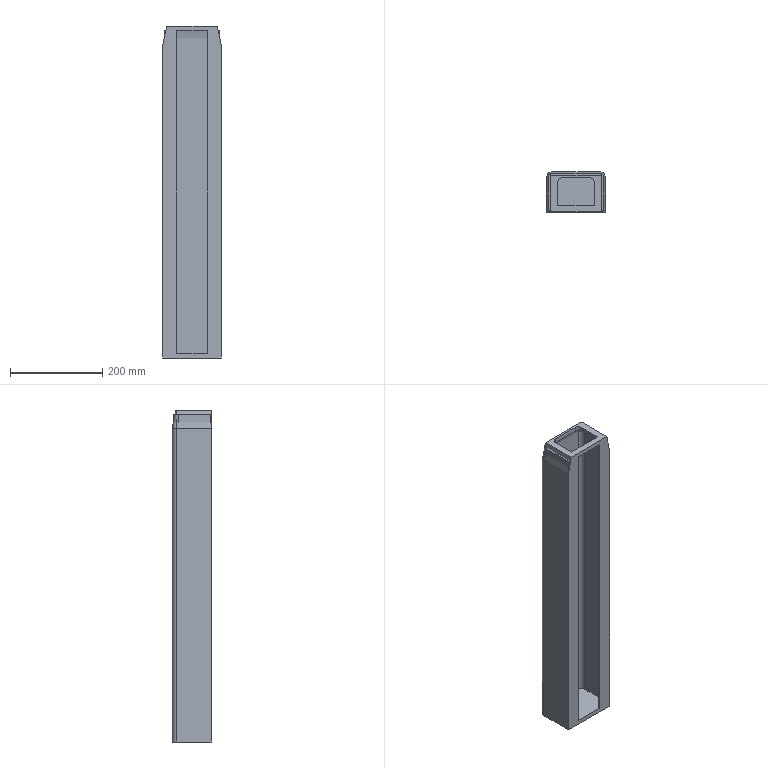Part | STEP file | 1 solid | 30 faces | box 126 x 86 x 720 mm | volume 848625 mm3 | plane 22 | cylinder 6 | cone 2 | commonest cylinder face diameters 20 x6